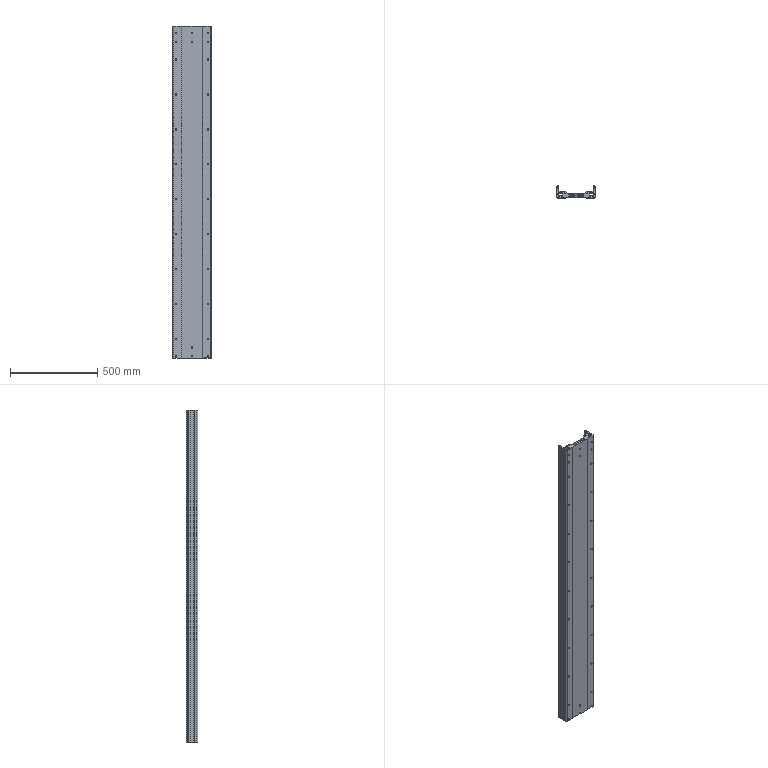Part | SolidWorks | features BaseBody 1 | 1 solid | 335 faces | box 220 x 67.5 x 1900 mm | volume 10276544 mm3 | cylinder 199 | plane 120 | cone 16 | commonest cylinder face diameters 8.6 x48 15 x48 4.3 x24 0.4 x20 6 x18 4.4 x12